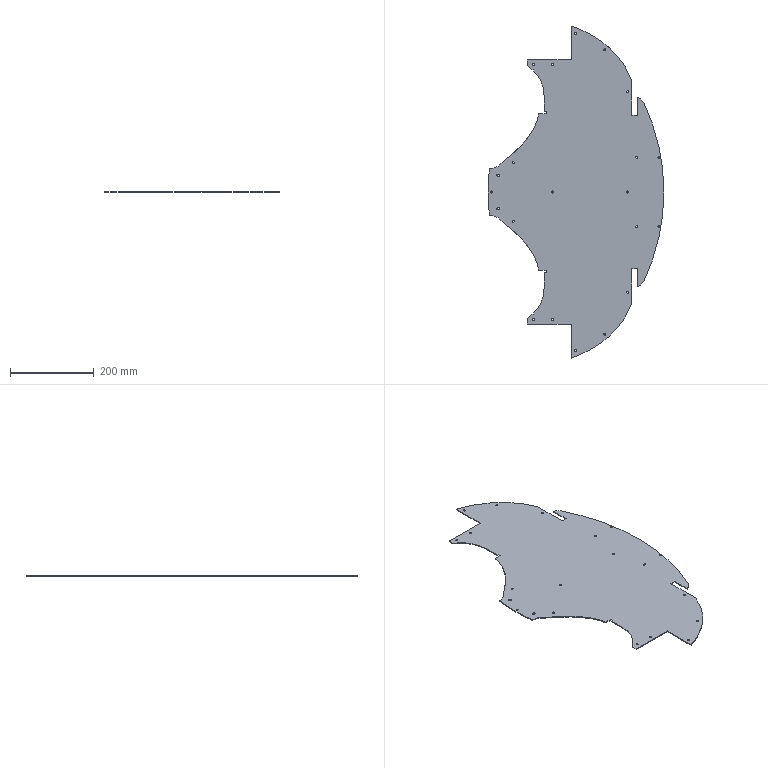Part | STEP file | Rear Consen Cover | 1 solid | 73 faces | box 420.328 x 794.391 x 2 mm | volume 399134 mm3 | cylinder 35 | plane 24 | spline 14 | commonest cylinder face diameters 5 x19 4 x2 6 x2 39.948 x2 47.766 x2 155.188 x2